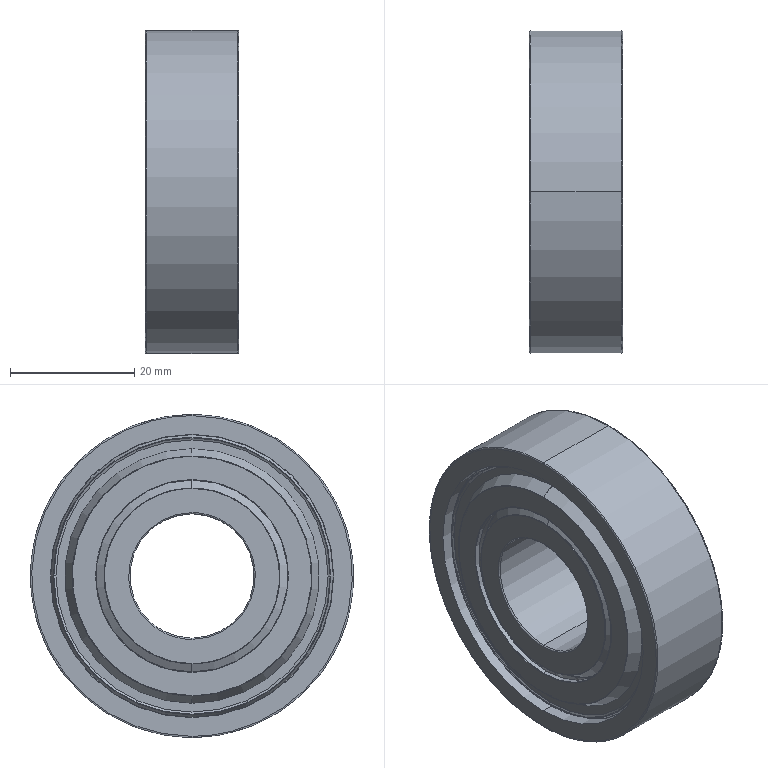Part | SolidWorks | features BaseBody 1 | 1 solid | 132 faces | box 15 x 52 x 52 mm | volume 22282 mm3 | spline 52 | cone 36 | cylinder 32 | plane 12 | commonest cylinder face diameters 31.2 x8 26.4 x4 28.32 x4 30.9 x4 40.8 x4 45.6 x4